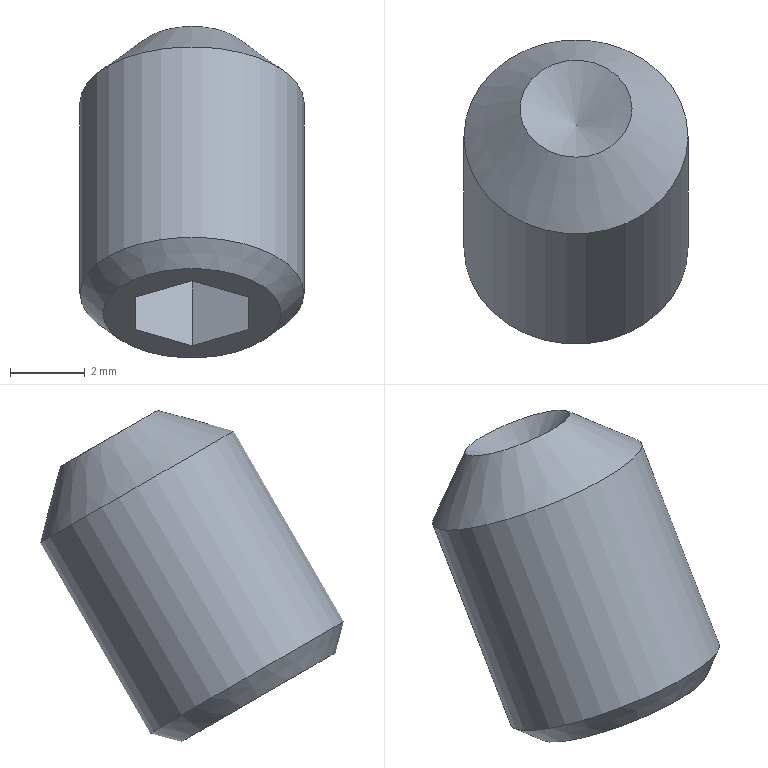Part | NX | features 5003_333_MSSU6-8 2 | 1 solid | 12 faces | box 6 x 8.139 x 8.871 mm | volume 187.509 mm3 | plane 8 | cone 3 | cylinder 1 | commonest cylinder face diameters 6 x1
STEP:
#1=CARTESIAN_POINT('',(1.025,114.25,-162.155));
#2=VERTEX_POINT('',#1);
#3=CARTESIAN_POINT('',(-0.475,113.5,-161.722));
#4=VERTEX_POINT('',#3);
#5=CARTESIAN_POINT('',(1.025,114.25,-162.155));
#6=DIRECTION('',(-0.866,-0.433,0.25));
#7=VECTOR('',#6,1000.);
#8=LINE('',#5,#7);
#9=EDGE_CURVE('',#2,#4,#8,.T.);
#10=ORIENTED_EDGE('',*,*,#9,.F.);
#11=CARTESIAN_POINT('',(1.025,115.75,-163.021));
#12=VERTEX_POINT('',#11);
#13=CARTESIAN_POINT('',(1.025,115.75,-163.021));
#14=DIRECTION('',(0.,-0.866,0.5));
#15=VECTOR('',#14,1000.);
#16=LINE('',#13,#15);
#17=EDGE_CURVE('',#12,#2,#16,.T.);
#18=ORIENTED_EDGE('',*,*,#17,.F.);
#19=CARTESIAN_POINT('',(-0.475,116.5,-163.454));
#20=VERTEX_POINT('',#19);
#21=CARTESIAN_POINT('',(-0.475,116.5,-163.454));
#22=DIRECTION('',(0.866,-0.433,0.25));
#23=VECTOR('',#22,1000.);
#24=LINE('',#21,#23);
#25=EDGE_CURVE('',#20,#12,#24,.T.);
#26=ORIENTED_EDGE('',*,*,#25,.F.);
#27=CARTESIAN_POINT('',(-1.975,115.75,-163.021));
#28=VERTEX_POINT('',#27);
#29=CARTESIAN_POINT('',(-1.975,115.75,-163.021));
#30=DIRECTION('',(0.866,0.433,-0.25));
#31=VECTOR('',#30,1000.);
#32=LINE('',#29,#31);
#33=EDGE_CURVE('',#28,#20,#32,.T.);
#34=ORIENTED_EDGE('',*,*,#33,.F.);
#35=CARTESIAN_POINT('',(-1.975,114.25,-162.155));
#36=VERTEX_POINT('',#35);
#37=CARTESIAN_POINT('',(-1.975,114.25,-162.155));
#38=DIRECTION('',(0.,0.866,-0.5));
#39=VECTOR('',#38,1000.);
#40=LINE('',#37,#39);
#41=EDGE_CURVE('',#36,#28,#40,.T.);
#42=ORIENTED_EDGE('',*,*,#41,.F.);
#43=CARTESIAN_POINT('',(-0.475,113.5,-161.722));
#44=DIRECTION('',(-0.866,0.433,-0.25));
#45=VECTOR('',#44,1000.);
#46=LINE('',#43,#45);
#47=EDGE_CURVE('',#4,#36,#46,.T.);
#48=ORIENTED_EDGE('',*,*,#47,.F.);
#49=EDGE_LOOP('',(#10,#18,#26,#34,#42,#48));
#50=FACE_BOUND('',#49,.T.);
#51=CARTESIAN_POINT('',(1.912,115.,-162.588));
#52=VERTEX_POINT('',#51);
#53=CARTESIAN_POINT('',(-0.475,115.,-162.588));
#54=DIRECTION('',(0.,-0.5,-0.866));
#55=DIRECTION('',(1.,0.,0.));
#56=AXIS2_PLACEMENT_3D('',#53,#54,#55);
#57=CIRCLE('',#56,2.386);
#58=EDGE_CURVE('',#52,#52,#57,.T.);
#59=ORIENTED_EDGE('',*,*,#58,.T.);
#60=EDGE_LOOP('',(#59));
#61=FACE_BOUND('',#60,.T.);
#62=CARTESIAN_POINT('',(-0.475,117.067,-163.782));
#63=DIRECTION('',(0.,-0.5,-0.866));
#64=DIRECTION('',(1.,0.,0.));
#65=AXIS2_PLACEMENT_3D('',#62,#63,#64);
#66=PLANE('',#65);
#67=ADVANCED_FACE('',(#50,#61),#66,.T.);
#68=CARTESIAN_POINT('',(-0.475,117.701,-154.91));
#69=VERTEX_POINT('',#68);
#70=CARTESIAN_POINT('',(-0.475,119.,-155.66));
#71=DIRECTION('',(0.,0.5,0.866));
#72=DIRECTION('',(0.,-0.866,0.5));
#73=AXIS2_PLACEMENT_3D('',#70,#71,#72);
#74=CIRCLE('',#73,1.5);
#75=EDGE_CURVE('',#69,#69,#74,.T.);
#76=ORIENTED_EDGE('',*,*,#75,.F.);
#77=EDGE_LOOP('',(#76));
#78=FACE_BOUND('',#77,.T.);
#79=CARTESIAN_POINT('',(2.525,118.25,-156.959));
#80=VERTEX_POINT('',#79);
#81=CARTESIAN_POINT('',(-0.475,118.25,-156.959));
#82=DIRECTION('',(0.,-0.5,-0.866));
#83=DIRECTION('',(1.,0.,0.));
#84=AXIS2_PLACEMENT_3D('',#81,#82,#83);
#85=CIRCLE('',#84,3.);
#86=EDGE_CURVE('',#80,#80,#85,.T.);
#87=ORIENTED_EDGE('',*,*,#86,.F.);
#88=EDGE_LOOP('',(#87));
#89=FACE_BOUND('',#88,.T.);
#90=CARTESIAN_POINT('',(-0.475,118.25,-156.959));
#91=DIRECTION('',(0.,-0.5,-0.866));
#92=DIRECTION('',(1.,0.,0.));
#93=AXIS2_PLACEMENT_3D('',#90,#91,#92);
#94=CONICAL_SURFACE('',#93,3.,0.7854);
#95=ADVANCED_FACE('',(#78,#89),#94,.T.);
#96=ORIENTED_EDGE('',*,*,#86,.T.);
#97=EDGE_LOOP('',(#96));
#98=FACE_BOUND('',#97,.T.);
#99=CARTESIAN_POINT('',(2.525,115.307,-162.057));
#100=VERTEX_POINT('',#99);
#101=CARTESIAN_POINT('',(-0.475,115.307,-162.057));
#102=DIRECTION('',(0.,-0.5,-0.866));
#103=DIRECTION('',(1.,0.,0.));
#104=AXIS2_PLACEMENT_3D('',#101,#102,#103);
#105=CIRCLE('',#104,3.);
#106=EDGE_CURVE('',#100,#100,#105,.T.);
#107=ORIENTED_EDGE('',*,*,#106,.F.);
#108=EDGE_LOOP('',(#107));
#109=FACE_BOUND('',#108,.T.);
#110=CARTESIAN_POINT('',(-0.475,114.8,-162.935));
#111=DIRECTION('',(0.,-0.5,-0.866));
#112=DIRECTION('',(1.,0.,0.));
#113=AXIS2_PLACEMENT_3D('',#110,#111,#112);
#114=CYLINDRICAL_SURFACE('',#113,3.);
#115=ADVANCED_FACE('',(#98,#109),#114,.T.);
#116=ORIENTED_EDGE('',*,*,#106,.T.);
#117=EDGE_LOOP('',(#116));
#118=FACE_BOUND('',#117,.T.);
#119=ORIENTED_EDGE('',*,*,#58,.F.);
#120=EDGE_LOOP('',(#119));
#121=FACE_BOUND('',#120,.T.);
#122=CARTESIAN_POINT('',(-0.475,115.,-162.588));
#123=DIRECTION('',(0.,0.5,0.866));
#124=DIRECTION('',(-1.,0.,0.));
#125=AXIS2_PLACEMENT_3D('',#122,#123,#124);
#126=CONICAL_SURFACE('',#125,2.386,0.7854);
#127=ADVANCED_FACE('',(#118,#121),#126,.T.);
#128=ORIENTED_EDGE('',*,*,#9,.T.);
#129=CARTESIAN_POINT('',(-0.475,114.5,-159.99));
#130=VERTEX_POINT('',#129);
#131=CARTESIAN_POINT('',(-0.475,114.5,-159.99));
#132=DIRECTION('',(0.,-0.5,-0.866));
#133=VECTOR('',#132,1000.);
#134=LINE('',#131,#133);
#135=EDGE_CURVE('',#130,#4,#134,.T.);
#136=ORIENTED_EDGE('',*,*,#135,.F.);
#137=CARTESIAN_POINT('',(1.025,115.25,-160.423));
#138=VERTEX_POINT('',#137);
#139=CARTESIAN_POINT('',(1.025,115.25,-160.423));
#140=DIRECTION('',(-0.866,-0.433,0.25));
#141=VECTOR('',#140,1000.);
#142=LINE('',#139,#141);
#143=EDGE_CURVE('',#138,#130,#142,.T.);
#144=ORIENTED_EDGE('',*,*,#143,.F.);
#145=CARTESIAN_POINT('',(1.025,115.25,-160.423));
#146=DIRECTION('',(0.,-0.5,-0.866));
#147=VECTOR('',#146,1000.);
#148=LINE('',#145,#147);
#149=EDGE_CURVE('',#138,#2,#148,.T.);
#150=ORIENTED_EDGE('',*,*,#149,.T.);
#151=EDGE_LOOP('',(#128,#136,#144,#150));
#152=FACE_BOUND('',#151,.T.);
#153=CARTESIAN_POINT('',(1.025,115.25,-160.423));
#154=DIRECTION('',(0.5,-0.75,0.433));
#155=DIRECTION('',(0.866,0.433,-0.25));
#156=AXIS2_PLACEMENT_3D('',#153,#154,#155);
#157=PLANE('',#156);
#158=ADVANCED_FACE('',(#152),#157,.F.);
#159=ORIENTED_EDGE('',*,*,#17,.T.);
#160=ORIENTED_EDGE('',*,*,#149,.F.);
#161=CARTESIAN_POINT('',(1.025,116.75,-161.289));
#162=VERTEX_POINT('',#161);
#163=CARTESIAN_POINT('',(1.025,116.75,-161.289));
#164=DIRECTION('',(0.,-0.866,0.5));
#165=VECTOR('',#164,1000.);
#166=LINE('',#163,#165);
#167=EDGE_CURVE('',#162,#138,#166,.T.);
#168=ORIENTED_EDGE('',*,*,#167,.F.);
#169=CARTESIAN_POINT('',(1.025,116.75,-161.289));
#170=DIRECTION('',(0.,-0.5,-0.866));
#171=VECTOR('',#170,1000.);
#172=LINE('',#169,#171);
#173=EDGE_CURVE('',#162,#12,#172,.T.);
#174=ORIENTED_EDGE('',*,*,#173,.T.);
#175=EDGE_LOOP('',(#159,#160,#168,#174));
#176=FACE_BOUND('',#175,.T.);
#177=CARTESIAN_POINT('',(1.025,116.75,-161.289));
#178=DIRECTION('',(1.,0.,0.));
#179=DIRECTION('',(0.,0.866,-0.5));
#180=AXIS2_PLACEMENT_3D('',#177,#178,#179);
#181=PLANE('',#180);
#182=ADVANCED_FACE('',(#176),#181,.F.);
#183=ORIENTED_EDGE('',*,*,#25,.T.);
#184=ORIENTED_EDGE('',*,*,#173,.F.);
#185=CARTESIAN_POINT('',(-0.475,117.5,-161.722));
#186=VERTEX_POINT('',#185);
#187=CARTESIAN_POINT('',(-0.475,117.5,-161.722));
#188=DIRECTION('',(0.866,-0.433,0.25));
#189=VECTOR('',#188,1000.);
#190=LINE('',#187,#189);
#191=EDGE_CURVE('',#186,#162,#190,.T.);
#192=ORIENTED_EDGE('',*,*,#191,.F.);
#193=CARTESIAN_POINT('',(-0.475,117.5,-161.722));
#194=DIRECTION('',(0.,-0.5,-0.866));
#195=VECTOR('',#194,1000.);
#196=LINE('',#193,#195);
#197=EDGE_CURVE('',#186,#20,#196,.T.);
#198=ORIENTED_EDGE('',*,*,#197,.T.);
#199=EDGE_LOOP('',(#183,#184,#192,#198));
#200=FACE_BOUND('',#199,.T.);
#201=CARTESIAN_POINT('',(-0.475,117.5,-161.722));
#202=DIRECTION('',(0.5,0.75,-0.433));
#203=DIRECTION('',(-0.866,0.433,-0.25));
#204=AXIS2_PLACEMENT_3D('',#201,#202,#203);
#205=PLANE('',#204);
#206=ADVANCED_FACE('',(#200),#205,.F.);
#207=ORIENTED_EDGE('',*,*,#33,.T.);
#208=ORIENTED_EDGE('',*,*,#197,.F.);
#209=CARTESIAN_POINT('',(-1.975,116.75,-161.289));
#210=VERTEX_POINT('',#209);
#211=CARTESIAN_POINT('',(-1.975,116.75,-161.289));
#212=DIRECTION('',(0.866,0.433,-0.25));
#213=VECTOR('',#212,1000.);
#214=LINE('',#211,#213);
#215=EDGE_CURVE('',#210,#186,#214,.T.);
#216=ORIENTED_EDGE('',*,*,#215,.F.);
#217=CARTESIAN_POINT('',(-1.975,116.75,-161.289));
#218=DIRECTION('',(0.,-0.5,-0.866));
#219=VECTOR('',#218,1000.);
#220=LINE('',#217,#219);
#221=EDGE_CURVE('',#210,#28,#220,.T.);
#222=ORIENTED_EDGE('',*,*,#221,.T.);
#223=EDGE_LOOP('',(#207,#208,#216,#222));
#224=FACE_BOUND('',#223,.T.);
#225=CARTESIAN_POINT('',(-1.975,116.75,-161.289));
#226=DIRECTION('',(-0.5,0.75,-0.433));
#227=DIRECTION('',(-0.866,-0.433,0.25));
#228=AXIS2_PLACEMENT_3D('',#225,#226,#227);
#229=PLANE('',#228);
#230=ADVANCED_FACE('',(#224),#229,.F.);
#231=ORIENTED_EDGE('',*,*,#41,.T.);
#232=ORIENTED_EDGE('',*,*,#221,.F.);
#233=CARTESIAN_POINT('',(-1.975,115.25,-160.423));
#234=VERTEX_POINT('',#233);
#235=CARTESIAN_POINT('',(-1.975,115.25,-160.423));
#236=DIRECTION('',(0.,0.866,-0.5));
#237=VECTOR('',#236,1000.);
#238=LINE('',#235,#237);
#239=EDGE_CURVE('',#234,#210,#238,.T.);
#240=ORIENTED_EDGE('',*,*,#239,.F.);
#241=CARTESIAN_POINT('',(-1.975,115.25,-160.423));
#242=DIRECTION('',(0.,-0.5,-0.866));
#243=VECTOR('',#242,1000.);
#244=LINE('',#241,#243);
#245=EDGE_CURVE('',#234,#36,#244,.T.);
#246=ORIENTED_EDGE('',*,*,#245,.T.);
#247=EDGE_LOOP('',(#231,#232,#240,#246));
#248=FACE_BOUND('',#247,.T.);
#249=CARTESIAN_POINT('',(-1.975,115.25,-160.423));
#250=DIRECTION('',(-1.,0.,0.));
#251=DIRECTION('',(0.,-0.5,-0.866));
#252=AXIS2_PLACEMENT_3D('',#249,#250,#251);
#253=PLANE('',#252);
#254=ADVANCED_FACE('',(#248),#253,.F.);
#255=ORIENTED_EDGE('',*,*,#47,.T.);
#256=ORIENTED_EDGE('',*,*,#245,.F.);
#257=CARTESIAN_POINT('',(-0.475,114.5,-159.99));
#258=DIRECTION('',(-0.866,0.433,-0.25));
#259=VECTOR('',#258,1000.);
#260=LINE('',#257,#259);
#261=EDGE_CURVE('',#130,#234,#260,.T.);
#262=ORIENTED_EDGE('',*,*,#261,.F.);
#263=ORIENTED_EDGE('',*,*,#135,.T.);
#264=EDGE_LOOP('',(#255,#256,#262,#263));
#265=FACE_BOUND('',#264,.T.);
#266=CARTESIAN_POINT('',(-0.475,114.5,-159.99));
#267=DIRECTION('',(-0.5,-0.75,0.433));
#268=DIRECTION('',(0.866,-0.433,0.25));
#269=AXIS2_PLACEMENT_3D('',#266,#267,#268);
#270=PLANE('',#269);
#271=ADVANCED_FACE('',(#265),#270,.F.);
#272=ORIENTED_EDGE('',*,*,#143,.T.);
#273=ORIENTED_EDGE('',*,*,#261,.T.);
#274=ORIENTED_EDGE('',*,*,#239,.T.);
#275=ORIENTED_EDGE('',*,*,#215,.T.);
#276=ORIENTED_EDGE('',*,*,#191,.T.);
#277=ORIENTED_EDGE('',*,*,#167,.T.);
#278=EDGE_LOOP('',(#272,#273,#274,#275,#276,#277));
#279=FACE_BOUND('',#278,.T.);
#280=CARTESIAN_POINT('',(-0.475,116.,-160.856));
#281=DIRECTION('',(0.,-0.5,-0.866));
#282=DIRECTION('',(1.,0.,0.));
#283=AXIS2_PLACEMENT_3D('',#280,#281,#282);
#284=PLANE('',#283);
#285=ADVANCED_FACE('',(#279),#284,.T.);
#286=ORIENTED_EDGE('',*,*,#75,.T.);
#287=EDGE_LOOP('',(#286));
#288=FACE_BOUND('',#287,.T.);
#289=CARTESIAN_POINT('',(-0.475,118.55,-156.44));
#290=VERTEX_POINT('',#289);
#291=VERTEX_LOOP('',#290);
#292=FACE_BOUND('',#291,.T.);
#293=CARTESIAN_POINT('',(-0.475,118.55,-156.44));
#294=DIRECTION('',(0.,0.5,0.866));
#295=DIRECTION('',(0.,-0.866,0.5));
#296=AXIS2_PLACEMENT_3D('',#293,#294,#295);
#297=CONICAL_SURFACE('',#296,0.,1.03);
#298=ADVANCED_FACE('',(#288,#292),#297,.F.);
#299=CLOSED_SHELL('',(#67,#95,#115,#127,#158,#182,#206,#230,#254,#271,#285,#298));
#300=MANIFOLD_SOLID_BREP('',#299);
#301=(LENGTH_UNIT()NAMED_UNIT(*)SI_UNIT(.MILLI.,.METRE.));
#302=UNCERTAINTY_MEASURE_WITH_UNIT(LENGTH_MEASURE(0.00001),#301,'','');
#303=(NAMED_UNIT(*)PLANE_ANGLE_UNIT()SI_UNIT($,.RADIAN.));
#304=(NAMED_UNIT(*)SI_UNIT($,.STERADIAN.)SOLID_ANGLE_UNIT());
#305=(GEOMETRIC_REPRESENTATION_CONTEXT(3)GLOBAL_UNCERTAINTY_ASSIGNED_CONTEXT((#302))GLOBAL_UNIT_ASSIGNED_CONTEXT((#301,#303,#304))REPRESENTATION_CONTEXT('',''));
#306=ADVANCED_BREP_SHAPE_REPRESENTATION('',(#300),#305);